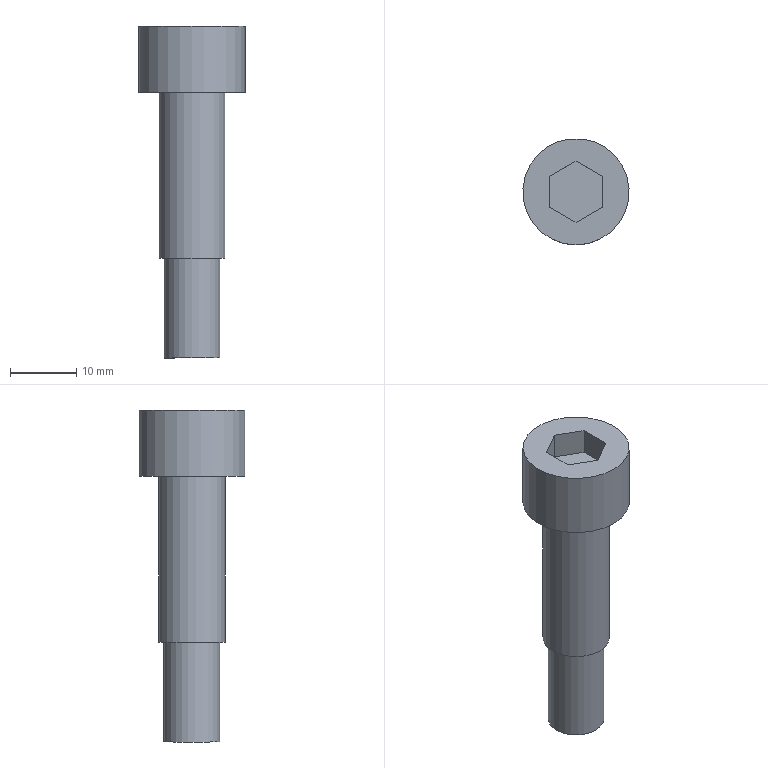Part | STEP file | CB-_id1534_x_t | 1 solid | 14 faces | box 16 x 16 x 50 mm | volume 4584 mm3 | plane 11 | cylinder 3 | commonest cylinder face diameters 8.4 x1 10 x1 16 x1
STEP:
#1=CARTESIAN_POINT('',(130.,232.2,-47.));
#2=VERTEX_POINT('',#1);
#3=CARTESIAN_POINT('',(130.,228.,-47.));
#4=DIRECTION('',(0.,0.,-1.));
#5=DIRECTION('',(0.,1.,0.));
#6=AXIS2_PLACEMENT_3D('',#3,#4,#5);
#7=CIRCLE('',#6,4.2);
#8=EDGE_CURVE('',#2,#2,#7,.T.);
#9=ORIENTED_EDGE('',*,*,#8,.F.);
#10=EDGE_LOOP('',(#9));
#11=FACE_BOUND('',#10,.T.);
#12=CARTESIAN_POINT('',(130.,223.,-47.));
#13=VERTEX_POINT('',#12);
#14=CARTESIAN_POINT('',(130.,228.,-47.));
#15=DIRECTION('',(0.,0.,1.));
#16=DIRECTION('',(0.,-1.,0.));
#17=AXIS2_PLACEMENT_3D('',#14,#15,#16);
#18=CIRCLE('',#17,5.);
#19=EDGE_CURVE('',#13,#13,#18,.T.);
#20=ORIENTED_EDGE('',*,*,#19,.F.);
#21=EDGE_LOOP('',(#20));
#22=FACE_BOUND('',#21,.T.);
#23=CARTESIAN_POINT('',(130.,228.,-47.));
#24=DIRECTION('',(0.,0.,-1.));
#25=DIRECTION('',(0.,1.,0.));
#26=AXIS2_PLACEMENT_3D('',#23,#24,#25);
#27=PLANE('',#26);
#28=ADVANCED_FACE('',(#11,#22),#27,.T.);
#29=CARTESIAN_POINT('',(130.,233.,-22.));
#30=VERTEX_POINT('',#29);
#31=CARTESIAN_POINT('',(130.,228.,-22.));
#32=DIRECTION('',(0.,0.,1.));
#33=DIRECTION('',(0.,1.,0.));
#34=AXIS2_PLACEMENT_3D('',#31,#32,#33);
#35=CIRCLE('',#34,5.);
#36=EDGE_CURVE('',#30,#30,#35,.T.);
#37=ORIENTED_EDGE('',*,*,#36,.F.);
#38=EDGE_LOOP('',(#37));
#39=FACE_BOUND('',#38,.T.);
#40=ORIENTED_EDGE('',*,*,#19,.T.);
#41=EDGE_LOOP('',(#40));
#42=FACE_BOUND('',#41,.T.);
#43=CARTESIAN_POINT('',(130.,228.,-47.));
#44=DIRECTION('',(0.,0.,1.));
#45=DIRECTION('',(0.,-1.,0.));
#46=AXIS2_PLACEMENT_3D('',#43,#44,#45);
#47=CYLINDRICAL_SURFACE('',#46,5.);
#48=ADVANCED_FACE('',(#39,#42),#47,.T.);
#49=CARTESIAN_POINT('',(130.,223.8,-62.));
#50=VERTEX_POINT('',#49);
#51=CARTESIAN_POINT('',(130.,228.,-62.));
#52=DIRECTION('',(0.,0.,1.));
#53=DIRECTION('',(0.,-1.,0.));
#54=AXIS2_PLACEMENT_3D('',#51,#52,#53);
#55=CIRCLE('',#54,4.2);
#56=EDGE_CURVE('',#50,#50,#55,.T.);
#57=ORIENTED_EDGE('',*,*,#56,.F.);
#58=EDGE_LOOP('',(#57));
#59=FACE_OUTER_BOUND('',#58,.T.);
#60=CARTESIAN_POINT('',(130.,228.,-62.));
#61=DIRECTION('',(0.,0.,-1.));
#62=DIRECTION('',(0.,1.,0.));
#63=AXIS2_PLACEMENT_3D('',#60,#61,#62);
#64=PLANE('',#63);
#65=ADVANCED_FACE('',(#59),#64,.T.);
#66=ORIENTED_EDGE('',*,*,#56,.T.);
#67=EDGE_LOOP('',(#66));
#68=FACE_BOUND('',#67,.T.);
#69=ORIENTED_EDGE('',*,*,#8,.T.);
#70=EDGE_LOOP('',(#69));
#71=FACE_BOUND('',#70,.T.);
#72=CARTESIAN_POINT('',(130.,228.,-47.));
#73=DIRECTION('',(0.,0.,-1.));
#74=DIRECTION('',(0.,-1.,0.));
#75=AXIS2_PLACEMENT_3D('',#72,#73,#74);
#76=CYLINDRICAL_SURFACE('',#75,4.2);
#77=ADVANCED_FACE('',(#68,#71),#76,.T.);
#78=CARTESIAN_POINT('',(134.,225.691,-12.));
#79=VERTEX_POINT('',#78);
#80=CARTESIAN_POINT('',(134.,230.309,-12.));
#81=VERTEX_POINT('',#80);
#82=CARTESIAN_POINT('',(134.,228.,-12.));
#83=DIRECTION('',(0.,1.,0.));
#84=VECTOR('',#83,1.);
#85=LINE('',#82,#84);
#86=EDGE_CURVE('',#79,#81,#85,.T.);
#87=ORIENTED_EDGE('',*,*,#86,.F.);
#88=CARTESIAN_POINT('',(130.,223.381,-12.));
#89=VERTEX_POINT('',#88);
#90=CARTESIAN_POINT('',(132.,224.536,-12.));
#91=DIRECTION('',(0.866,0.5,0.));
#92=VECTOR('',#91,1.);
#93=LINE('',#90,#92);
#94=EDGE_CURVE('',#89,#79,#93,.T.);
#95=ORIENTED_EDGE('',*,*,#94,.F.);
#96=CARTESIAN_POINT('',(126.,225.691,-12.));
#97=VERTEX_POINT('',#96);
#98=CARTESIAN_POINT('',(128.,224.536,-12.));
#99=DIRECTION('',(0.866,-0.5,0.));
#100=VECTOR('',#99,1.);
#101=LINE('',#98,#100);
#102=EDGE_CURVE('',#97,#89,#101,.T.);
#103=ORIENTED_EDGE('',*,*,#102,.F.);
#104=CARTESIAN_POINT('',(126.,230.309,-12.));
#105=VERTEX_POINT('',#104);
#106=CARTESIAN_POINT('',(126.,228.,-12.));
#107=DIRECTION('',(0.,-1.,0.));
#108=VECTOR('',#107,1.);
#109=LINE('',#106,#108);
#110=EDGE_CURVE('',#105,#97,#109,.T.);
#111=ORIENTED_EDGE('',*,*,#110,.F.);
#112=CARTESIAN_POINT('',(130.,232.619,-12.));
#113=VERTEX_POINT('',#112);
#114=CARTESIAN_POINT('',(128.,231.464,-12.));
#115=DIRECTION('',(-0.866,-0.5,0.));
#116=VECTOR('',#115,1.);
#117=LINE('',#114,#116);
#118=EDGE_CURVE('',#113,#105,#117,.T.);
#119=ORIENTED_EDGE('',*,*,#118,.F.);
#120=CARTESIAN_POINT('',(132.,231.464,-12.));
#121=DIRECTION('',(-0.866,0.5,0.));
#122=VECTOR('',#121,1.);
#123=LINE('',#120,#122);
#124=EDGE_CURVE('',#81,#113,#123,.T.);
#125=ORIENTED_EDGE('',*,*,#124,.F.);
#126=EDGE_LOOP('',(#87,#95,#103,#111,#119,#125));
#127=FACE_BOUND('',#126,.T.);
#128=CARTESIAN_POINT('',(130.,220.,-12.));
#129=VERTEX_POINT('',#128);
#130=CARTESIAN_POINT('',(130.,228.,-12.));
#131=DIRECTION('',(0.,0.,-1.));
#132=DIRECTION('',(0.,-1.,0.));
#133=AXIS2_PLACEMENT_3D('',#130,#131,#132);
#134=CIRCLE('',#133,8.);
#135=EDGE_CURVE('',#129,#129,#134,.T.);
#136=ORIENTED_EDGE('',*,*,#135,.F.);
#137=EDGE_LOOP('',(#136));
#138=FACE_BOUND('',#137,.T.);
#139=CARTESIAN_POINT('',(130.,228.,-12.));
#140=DIRECTION('',(0.,0.,1.));
#141=DIRECTION('',(0.,-1.,0.));
#142=AXIS2_PLACEMENT_3D('',#139,#140,#141);
#143=PLANE('',#142);
#144=ADVANCED_FACE('',(#127,#138),#143,.T.);
#145=ORIENTED_EDGE('',*,*,#36,.T.);
#146=EDGE_LOOP('',(#145));
#147=FACE_BOUND('',#146,.T.);
#148=CARTESIAN_POINT('',(130.,220.,-22.));
#149=VERTEX_POINT('',#148);
#150=CARTESIAN_POINT('',(130.,228.,-22.));
#151=DIRECTION('',(0.,0.,1.));
#152=DIRECTION('',(0.,-1.,0.));
#153=AXIS2_PLACEMENT_3D('',#150,#151,#152);
#154=CIRCLE('',#153,8.);
#155=EDGE_CURVE('',#149,#149,#154,.T.);
#156=ORIENTED_EDGE('',*,*,#155,.F.);
#157=EDGE_LOOP('',(#156));
#158=FACE_BOUND('',#157,.T.);
#159=CARTESIAN_POINT('',(130.,228.,-22.));
#160=DIRECTION('',(0.,0.,-1.));
#161=DIRECTION('',(0.,1.,0.));
#162=AXIS2_PLACEMENT_3D('',#159,#160,#161);
#163=PLANE('',#162);
#164=ADVANCED_FACE('',(#147,#158),#163,.T.);
#165=ORIENTED_EDGE('',*,*,#135,.T.);
#166=EDGE_LOOP('',(#165));
#167=FACE_BOUND('',#166,.T.);
#168=ORIENTED_EDGE('',*,*,#155,.T.);
#169=EDGE_LOOP('',(#168));
#170=FACE_BOUND('',#169,.T.);
#171=CARTESIAN_POINT('',(130.,228.,-22.));
#172=DIRECTION('',(0.,0.,1.));
#173=DIRECTION('',(0.,-1.,0.));
#174=AXIS2_PLACEMENT_3D('',#171,#172,#173);
#175=CYLINDRICAL_SURFACE('',#174,8.);
#176=ADVANCED_FACE('',(#167,#170),#175,.T.);
#177=ORIENTED_EDGE('',*,*,#86,.T.);
#178=CARTESIAN_POINT('',(134.,230.309,-16.));
#179=VERTEX_POINT('',#178);
#180=CARTESIAN_POINT('',(134.,230.309,-70.5));
#181=DIRECTION('',(0.,0.,-1.));
#182=VECTOR('',#181,1.);
#183=LINE('',#180,#182);
#184=EDGE_CURVE('',#81,#179,#183,.T.);
#185=ORIENTED_EDGE('',*,*,#184,.T.);
#186=CARTESIAN_POINT('',(134.,225.691,-16.));
#187=VERTEX_POINT('',#186);
#188=CARTESIAN_POINT('',(134.,228.,-16.));
#189=DIRECTION('',(0.,-1.,0.));
#190=VECTOR('',#189,1.);
#191=LINE('',#188,#190);
#192=EDGE_CURVE('',#179,#187,#191,.T.);
#193=ORIENTED_EDGE('',*,*,#192,.T.);
#194=CARTESIAN_POINT('',(134.,225.691,-70.5));
#195=DIRECTION('',(0.,0.,-1.));
#196=VECTOR('',#195,1.);
#197=LINE('',#194,#196);
#198=EDGE_CURVE('',#79,#187,#197,.T.);
#199=ORIENTED_EDGE('',*,*,#198,.F.);
#200=EDGE_LOOP('',(#177,#185,#193,#199));
#201=FACE_OUTER_BOUND('',#200,.T.);
#202=CARTESIAN_POINT('',(134.,228.,-70.5));
#203=DIRECTION('',(1.,0.,0.));
#204=DIRECTION('',(0.,0.,-1.));
#205=AXIS2_PLACEMENT_3D('',#202,#203,#204);
#206=PLANE('',#205);
#207=ADVANCED_FACE('',(#201),#206,.F.);
#208=ORIENTED_EDGE('',*,*,#94,.T.);
#209=ORIENTED_EDGE('',*,*,#198,.T.);
#210=CARTESIAN_POINT('',(130.,223.381,-16.));
#211=VERTEX_POINT('',#210);
#212=CARTESIAN_POINT('',(132.,224.536,-16.));
#213=DIRECTION('',(-0.866,-0.5,0.));
#214=VECTOR('',#213,1.);
#215=LINE('',#212,#214);
#216=EDGE_CURVE('',#187,#211,#215,.T.);
#217=ORIENTED_EDGE('',*,*,#216,.T.);
#218=CARTESIAN_POINT('',(130.,223.381,-70.5));
#219=DIRECTION('',(0.,0.,-1.));
#220=VECTOR('',#219,1.);
#221=LINE('',#218,#220);
#222=EDGE_CURVE('',#89,#211,#221,.T.);
#223=ORIENTED_EDGE('',*,*,#222,.F.);
#224=EDGE_LOOP('',(#208,#209,#217,#223));
#225=FACE_OUTER_BOUND('',#224,.T.);
#226=CARTESIAN_POINT('',(132.,224.536,-70.5));
#227=DIRECTION('',(0.5,-0.866,0.));
#228=DIRECTION('',(0.866,0.5,0.));
#229=AXIS2_PLACEMENT_3D('',#226,#227,#228);
#230=PLANE('',#229);
#231=ADVANCED_FACE('',(#225),#230,.F.);
#232=ORIENTED_EDGE('',*,*,#102,.T.);
#233=ORIENTED_EDGE('',*,*,#222,.T.);
#234=CARTESIAN_POINT('',(126.,225.691,-16.));
#235=VERTEX_POINT('',#234);
#236=CARTESIAN_POINT('',(128.,224.536,-16.));
#237=DIRECTION('',(-0.866,0.5,0.));
#238=VECTOR('',#237,1.);
#239=LINE('',#236,#238);
#240=EDGE_CURVE('',#211,#235,#239,.T.);
#241=ORIENTED_EDGE('',*,*,#240,.T.);
#242=CARTESIAN_POINT('',(126.,225.691,-70.5));
#243=DIRECTION('',(0.,0.,-1.));
#244=VECTOR('',#243,1.);
#245=LINE('',#242,#244);
#246=EDGE_CURVE('',#97,#235,#245,.T.);
#247=ORIENTED_EDGE('',*,*,#246,.F.);
#248=EDGE_LOOP('',(#232,#233,#241,#247));
#249=FACE_OUTER_BOUND('',#248,.T.);
#250=CARTESIAN_POINT('',(128.,224.536,-70.5));
#251=DIRECTION('',(-0.5,-0.866,0.));
#252=DIRECTION('',(0.866,-0.5,0.));
#253=AXIS2_PLACEMENT_3D('',#250,#251,#252);
#254=PLANE('',#253);
#255=ADVANCED_FACE('',(#249),#254,.F.);
#256=ORIENTED_EDGE('',*,*,#110,.T.);
#257=ORIENTED_EDGE('',*,*,#246,.T.);
#258=CARTESIAN_POINT('',(126.,230.309,-16.));
#259=VERTEX_POINT('',#258);
#260=CARTESIAN_POINT('',(126.,228.,-16.));
#261=DIRECTION('',(0.,1.,0.));
#262=VECTOR('',#261,1.);
#263=LINE('',#260,#262);
#264=EDGE_CURVE('',#235,#259,#263,.T.);
#265=ORIENTED_EDGE('',*,*,#264,.T.);
#266=CARTESIAN_POINT('',(126.,230.309,-70.5));
#267=DIRECTION('',(0.,0.,-1.));
#268=VECTOR('',#267,1.);
#269=LINE('',#266,#268);
#270=EDGE_CURVE('',#105,#259,#269,.T.);
#271=ORIENTED_EDGE('',*,*,#270,.F.);
#272=EDGE_LOOP('',(#256,#257,#265,#271));
#273=FACE_OUTER_BOUND('',#272,.T.);
#274=CARTESIAN_POINT('',(126.,228.,-70.5));
#275=DIRECTION('',(-1.,0.,0.));
#276=DIRECTION('',(0.,0.,1.));
#277=AXIS2_PLACEMENT_3D('',#274,#275,#276);
#278=PLANE('',#277);
#279=ADVANCED_FACE('',(#273),#278,.F.);
#280=ORIENTED_EDGE('',*,*,#118,.T.);
#281=ORIENTED_EDGE('',*,*,#270,.T.);
#282=CARTESIAN_POINT('',(130.,232.619,-16.));
#283=VERTEX_POINT('',#282);
#284=CARTESIAN_POINT('',(128.,231.464,-16.));
#285=DIRECTION('',(0.866,0.5,0.));
#286=VECTOR('',#285,1.);
#287=LINE('',#284,#286);
#288=EDGE_CURVE('',#259,#283,#287,.T.);
#289=ORIENTED_EDGE('',*,*,#288,.T.);
#290=CARTESIAN_POINT('',(130.,232.619,-70.5));
#291=DIRECTION('',(0.,0.,-1.));
#292=VECTOR('',#291,1.);
#293=LINE('',#290,#292);
#294=EDGE_CURVE('',#113,#283,#293,.T.);
#295=ORIENTED_EDGE('',*,*,#294,.F.);
#296=EDGE_LOOP('',(#280,#281,#289,#295));
#297=FACE_OUTER_BOUND('',#296,.T.);
#298=CARTESIAN_POINT('',(128.,231.464,-70.5));
#299=DIRECTION('',(-0.5,0.866,0.));
#300=DIRECTION('',(-0.866,-0.5,0.));
#301=AXIS2_PLACEMENT_3D('',#298,#299,#300);
#302=PLANE('',#301);
#303=ADVANCED_FACE('',(#297),#302,.F.);
#304=ORIENTED_EDGE('',*,*,#124,.T.);
#305=ORIENTED_EDGE('',*,*,#294,.T.);
#306=CARTESIAN_POINT('',(132.,231.464,-16.));
#307=DIRECTION('',(0.866,-0.5,0.));
#308=VECTOR('',#307,1.);
#309=LINE('',#306,#308);
#310=EDGE_CURVE('',#283,#179,#309,.T.);
#311=ORIENTED_EDGE('',*,*,#310,.T.);
#312=ORIENTED_EDGE('',*,*,#184,.F.);
#313=EDGE_LOOP('',(#304,#305,#311,#312));
#314=FACE_OUTER_BOUND('',#313,.T.);
#315=CARTESIAN_POINT('',(132.,231.464,-70.5));
#316=DIRECTION('',(0.5,0.866,0.));
#317=DIRECTION('',(-0.866,0.5,0.));
#318=AXIS2_PLACEMENT_3D('',#315,#316,#317);
#319=PLANE('',#318);
#320=ADVANCED_FACE('',(#314),#319,.F.);
#321=ORIENTED_EDGE('',*,*,#192,.F.);
#322=ORIENTED_EDGE('',*,*,#310,.F.);
#323=ORIENTED_EDGE('',*,*,#288,.F.);
#324=ORIENTED_EDGE('',*,*,#264,.F.);
#325=ORIENTED_EDGE('',*,*,#240,.F.);
#326=ORIENTED_EDGE('',*,*,#216,.F.);
#327=EDGE_LOOP('',(#321,#322,#323,#324,#325,#326));
#328=FACE_OUTER_BOUND('',#327,.T.);
#329=CARTESIAN_POINT('',(130.,228.,-16.));
#330=DIRECTION('',(0.,0.,1.));
#331=DIRECTION('',(0.,-1.,0.));
#332=AXIS2_PLACEMENT_3D('',#329,#330,#331);
#333=PLANE('',#332);
#334=ADVANCED_FACE('',(#328),#333,.T.);
#335=CLOSED_SHELL('',(#28,#48,#65,#77,#144,#164,#176,#207,#231,#255,#279,#303,#320,#334));
#336=MANIFOLD_SOLID_BREP('',#335);
#337=(LENGTH_UNIT()NAMED_UNIT(*)SI_UNIT(.MILLI.,.METRE.));
#338=UNCERTAINTY_MEASURE_WITH_UNIT(LENGTH_MEASURE(0.00002),#337,'','');
#339=(NAMED_UNIT(*)PLANE_ANGLE_UNIT()SI_UNIT($,.RADIAN.));
#340=PLANE_ANGLE_MEASURE_WITH_UNIT(PLANE_ANGLE_MEASURE(0.01745),#339);
#341=DIMENSIONAL_EXPONENTS(0.,0.,0.,0.,0.,0.,0.);
#342=(CONVERSION_BASED_UNIT('DEGREE',#340)NAMED_UNIT(#341)PLANE_ANGLE_UNIT());
#343=(NAMED_UNIT(*)SI_UNIT($,.STERADIAN.)SOLID_ANGLE_UNIT());
#344=(GEOMETRIC_REPRESENTATION_CONTEXT(3)GLOBAL_UNCERTAINTY_ASSIGNED_CONTEXT((#338))GLOBAL_UNIT_ASSIGNED_CONTEXT((#337,#342,#343))REPRESENTATION_CONTEXT('',''));
#345=ADVANCED_BREP_SHAPE_REPRESENTATION('',(#336),#344);